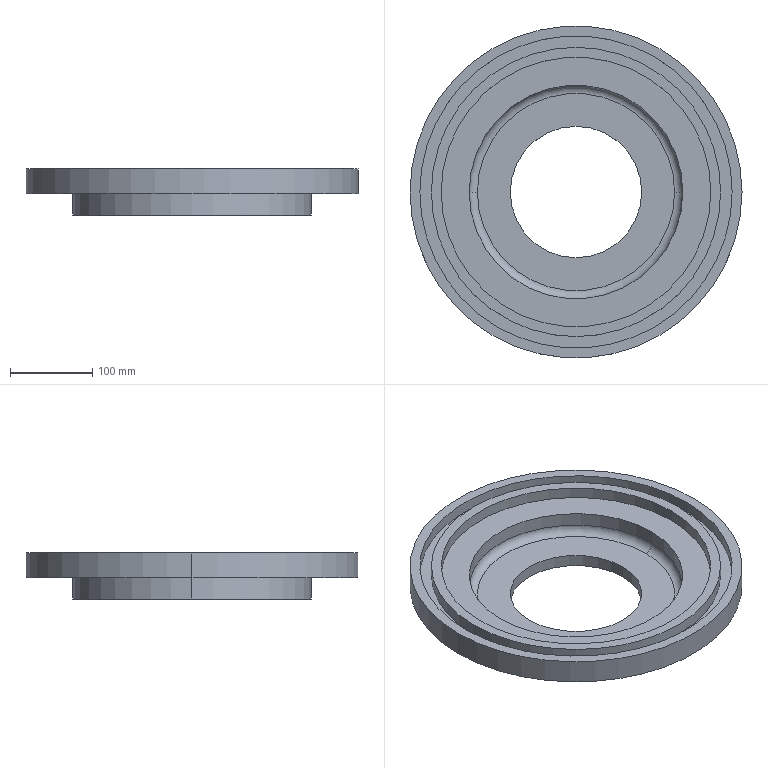Part | SolidWorks | features Fillet 1, Revolution 1 | 1 solid | 23 faces | box 404 x 404 x 56 mm | volume 2436851 mm3 | cylinder 14 | plane 7 | torus 2 | commonest cylinder face diameters 160 x2 260 x2 290 x2 328 x2 352 x2 380 x2
STEP:
#1=CARTESIAN_POINT('',(130.,0.,-31.));
#2=VERTEX_POINT('',#1);
#3=CARTESIAN_POINT('',(-130.,0.,-31.));
#4=VERTEX_POINT('',#3);
#5=CARTESIAN_POINT('',(0.,0.,-31.));
#6=DIRECTION('',(0.,0.,-1.));
#7=DIRECTION('',(-1.,0.,0.));
#8=AXIS2_PLACEMENT_3D('',#5,#6,#7);
#9=CIRCLE('',#8,130.);
#10=EDGE_CURVE('',#2,#4,#9,.T.);
#11=ORIENTED_EDGE('',*,*,#10,.F.);
#12=CARTESIAN_POINT('',(120.,0.,-41.));
#13=VERTEX_POINT('',#12);
#14=CARTESIAN_POINT('',(120.,0.,-31.));
#15=DIRECTION('',(0.,1.,0.));
#16=DIRECTION('',(-1.,0.,0.));
#17=AXIS2_PLACEMENT_3D('',#14,#15,#16);
#18=CIRCLE('',#17,10.);
#19=EDGE_CURVE('',#2,#13,#18,.T.);
#20=ORIENTED_EDGE('',*,*,#19,.T.);
#21=CARTESIAN_POINT('',(-120.,0.,-41.));
#22=VERTEX_POINT('',#21);
#23=CARTESIAN_POINT('',(0.,0.,-41.));
#24=DIRECTION('',(0.,0.,1.));
#25=DIRECTION('',(-1.,0.,0.));
#26=AXIS2_PLACEMENT_3D('',#23,#24,#25);
#27=CIRCLE('',#26,120.);
#28=EDGE_CURVE('',#22,#13,#27,.T.);
#29=ORIENTED_EDGE('',*,*,#28,.F.);
#30=CARTESIAN_POINT('',(-120.,0.,-31.));
#31=DIRECTION('',(0.,-1.,0.));
#32=DIRECTION('',(0.,0.,-1.));
#33=AXIS2_PLACEMENT_3D('',#30,#31,#32);
#34=CIRCLE('',#33,10.);
#35=EDGE_CURVE('',#4,#22,#34,.T.);
#36=ORIENTED_EDGE('',*,*,#35,.F.);
#37=EDGE_LOOP('',(#11,#20,#29,#36));
#38=FACE_OUTER_BOUND('',#37,.T.);
#39=CARTESIAN_POINT('',(0.,0.,-31.));
#40=DIRECTION('',(0.,0.,-1.));
#41=DIRECTION('',(-1.,0.,0.));
#42=AXIS2_PLACEMENT_3D('',#39,#40,#41);
#43=TOROIDAL_SURFACE('',#42,120.,10.);
#44=ADVANCED_FACE('',(#38),#43,.F.);
#45=CARTESIAN_POINT('',(-190.,0.,-14.));
#46=VERTEX_POINT('',#45);
#47=CARTESIAN_POINT('',(190.,0.,-14.));
#48=VERTEX_POINT('',#47);
#49=CARTESIAN_POINT('',(0.,0.,-14.));
#50=DIRECTION('',(0.,0.,1.));
#51=DIRECTION('',(1.,0.,0.));
#52=AXIS2_PLACEMENT_3D('',#49,#50,#51);
#53=CIRCLE('',#52,190.);
#54=EDGE_CURVE('',#46,#48,#53,.T.);
#55=ORIENTED_EDGE('',*,*,#54,.F.);
#56=CARTESIAN_POINT('',(-190.,0.,0.));
#57=VERTEX_POINT('',#56);
#58=CARTESIAN_POINT('',(-190.,0.,0.));
#59=DIRECTION('',(0.,0.,1.));
#60=VECTOR('',#59,1000.);
#61=LINE('',#58,#60);
#62=EDGE_CURVE('',#46,#57,#61,.T.);
#63=ORIENTED_EDGE('',*,*,#62,.T.);
#64=CARTESIAN_POINT('',(190.,0.,0.));
#65=VERTEX_POINT('',#64);
#66=CARTESIAN_POINT('',(0.,0.,0.));
#67=DIRECTION('',(0.,0.,1.));
#68=DIRECTION('',(1.,0.,0.));
#69=AXIS2_PLACEMENT_3D('',#66,#67,#68);
#70=CIRCLE('',#69,190.);
#71=EDGE_CURVE('',#57,#65,#70,.T.);
#72=ORIENTED_EDGE('',*,*,#71,.T.);
#73=CARTESIAN_POINT('',(190.,0.,0.));
#74=DIRECTION('',(0.,0.,1.));
#75=VECTOR('',#74,1000.);
#76=LINE('',#73,#75);
#77=EDGE_CURVE('',#48,#65,#76,.T.);
#78=ORIENTED_EDGE('',*,*,#77,.F.);
#79=EDGE_LOOP('',(#55,#63,#72,#78));
#80=FACE_OUTER_BOUND('',#79,.T.);
#81=CARTESIAN_POINT('',(0.,0.,0.));
#82=DIRECTION('',(0.,0.,1.));
#83=DIRECTION('',(1.,0.,0.));
#84=AXIS2_PLACEMENT_3D('',#81,#82,#83);
#85=CYLINDRICAL_SURFACE('',#84,190.);
#86=ADVANCED_FACE('',(#80),#85,.F.);
#87=CARTESIAN_POINT('',(176.,0.,-14.));
#88=VERTEX_POINT('',#87);
#89=CARTESIAN_POINT('',(-176.,0.,-14.));
#90=VERTEX_POINT('',#89);
#91=CARTESIAN_POINT('',(0.,0.,-14.));
#92=DIRECTION('',(0.,0.,1.));
#93=DIRECTION('',(1.,0.,0.));
#94=AXIS2_PLACEMENT_3D('',#91,#92,#93);
#95=CIRCLE('',#94,176.);
#96=EDGE_CURVE('',#88,#90,#95,.T.);
#97=ORIENTED_EDGE('',*,*,#96,.T.);
#98=CARTESIAN_POINT('',(-176.,0.,0.));
#99=VERTEX_POINT('',#98);
#100=CARTESIAN_POINT('',(-176.,0.,0.));
#101=DIRECTION('',(0.,0.,1.));
#102=VECTOR('',#101,1000.);
#103=LINE('',#100,#102);
#104=EDGE_CURVE('',#90,#99,#103,.T.);
#105=ORIENTED_EDGE('',*,*,#104,.T.);
#106=CARTESIAN_POINT('',(176.,0.,0.));
#107=VERTEX_POINT('',#106);
#108=CARTESIAN_POINT('',(0.,0.,0.));
#109=DIRECTION('',(0.,0.,1.));
#110=DIRECTION('',(1.,0.,0.));
#111=AXIS2_PLACEMENT_3D('',#108,#109,#110);
#112=CIRCLE('',#111,176.);
#113=EDGE_CURVE('',#107,#99,#112,.T.);
#114=ORIENTED_EDGE('',*,*,#113,.F.);
#115=CARTESIAN_POINT('',(176.,0.,0.));
#116=DIRECTION('',(0.,0.,1.));
#117=VECTOR('',#116,1000.);
#118=LINE('',#115,#117);
#119=EDGE_CURVE('',#88,#107,#118,.T.);
#120=ORIENTED_EDGE('',*,*,#119,.F.);
#121=EDGE_LOOP('',(#97,#105,#114,#120));
#122=FACE_OUTER_BOUND('',#121,.T.);
#123=CARTESIAN_POINT('',(0.,0.,0.));
#124=DIRECTION('',(0.,0.,1.));
#125=DIRECTION('',(1.,0.,0.));
#126=AXIS2_PLACEMENT_3D('',#123,#124,#125);
#127=CYLINDRICAL_SURFACE('',#126,176.);
#128=ADVANCED_FACE('',(#122),#127,.T.);
#129=CARTESIAN_POINT('',(-164.,0.,-14.));
#130=VERTEX_POINT('',#129);
#131=CARTESIAN_POINT('',(164.,0.,-14.));
#132=VERTEX_POINT('',#131);
#133=CARTESIAN_POINT('',(0.,0.,-14.));
#134=DIRECTION('',(0.,0.,1.));
#135=DIRECTION('',(1.,0.,0.));
#136=AXIS2_PLACEMENT_3D('',#133,#134,#135);
#137=CIRCLE('',#136,164.);
#138=EDGE_CURVE('',#130,#132,#137,.T.);
#139=ORIENTED_EDGE('',*,*,#138,.F.);
#140=CARTESIAN_POINT('',(-164.,0.,0.));
#141=VERTEX_POINT('',#140);
#142=CARTESIAN_POINT('',(-164.,0.,0.));
#143=DIRECTION('',(0.,0.,1.));
#144=VECTOR('',#143,1000.);
#145=LINE('',#142,#144);
#146=EDGE_CURVE('',#130,#141,#145,.T.);
#147=ORIENTED_EDGE('',*,*,#146,.T.);
#148=CARTESIAN_POINT('',(164.,0.,0.));
#149=VERTEX_POINT('',#148);
#150=CARTESIAN_POINT('',(0.,0.,0.));
#151=DIRECTION('',(0.,0.,1.));
#152=DIRECTION('',(1.,0.,0.));
#153=AXIS2_PLACEMENT_3D('',#150,#151,#152);
#154=CIRCLE('',#153,164.);
#155=EDGE_CURVE('',#141,#149,#154,.T.);
#156=ORIENTED_EDGE('',*,*,#155,.T.);
#157=CARTESIAN_POINT('',(164.,0.,0.));
#158=DIRECTION('',(0.,0.,1.));
#159=VECTOR('',#158,1000.);
#160=LINE('',#157,#159);
#161=EDGE_CURVE('',#132,#149,#160,.T.);
#162=ORIENTED_EDGE('',*,*,#161,.F.);
#163=EDGE_LOOP('',(#139,#147,#156,#162));
#164=FACE_OUTER_BOUND('',#163,.T.);
#165=CARTESIAN_POINT('',(0.,0.,0.));
#166=DIRECTION('',(0.,0.,1.));
#167=DIRECTION('',(1.,0.,0.));
#168=AXIS2_PLACEMENT_3D('',#165,#166,#167);
#169=CYLINDRICAL_SURFACE('',#168,164.);
#170=ADVANCED_FACE('',(#164),#169,.F.);
#171=ORIENTED_EDGE('',*,*,#10,.T.);
#172=CARTESIAN_POINT('',(-130.,0.,-14.));
#173=VERTEX_POINT('',#172);
#174=CARTESIAN_POINT('',(-130.,0.,0.));
#175=DIRECTION('',(0.,0.,1.));
#176=VECTOR('',#175,1000.);
#177=LINE('',#174,#176);
#178=EDGE_CURVE('',#4,#173,#177,.T.);
#179=ORIENTED_EDGE('',*,*,#178,.T.);
#180=CARTESIAN_POINT('',(130.,0.,-14.));
#181=VERTEX_POINT('',#180);
#182=CARTESIAN_POINT('',(0.,0.,-14.));
#183=DIRECTION('',(0.,0.,1.));
#184=DIRECTION('',(1.,0.,0.));
#185=AXIS2_PLACEMENT_3D('',#182,#183,#184);
#186=CIRCLE('',#185,130.);
#187=EDGE_CURVE('',#173,#181,#186,.T.);
#188=ORIENTED_EDGE('',*,*,#187,.T.);
#189=CARTESIAN_POINT('',(130.,0.,0.));
#190=DIRECTION('',(0.,0.,1.));
#191=VECTOR('',#190,1000.);
#192=LINE('',#189,#191);
#193=EDGE_CURVE('',#2,#181,#192,.T.);
#194=ORIENTED_EDGE('',*,*,#193,.F.);
#195=EDGE_LOOP('',(#171,#179,#188,#194));
#196=FACE_OUTER_BOUND('',#195,.T.);
#197=CARTESIAN_POINT('',(0.,0.,0.));
#198=DIRECTION('',(0.,0.,1.));
#199=DIRECTION('',(1.,0.,0.));
#200=AXIS2_PLACEMENT_3D('',#197,#198,#199);
#201=CYLINDRICAL_SURFACE('',#200,130.);
#202=ADVANCED_FACE('',(#196),#201,.F.);
#203=CARTESIAN_POINT('',(-80.,0.,-56.));
#204=VERTEX_POINT('',#203);
#205=CARTESIAN_POINT('',(80.,0.,-56.));
#206=VERTEX_POINT('',#205);
#207=CARTESIAN_POINT('',(0.,0.,-56.));
#208=DIRECTION('',(0.,0.,1.));
#209=DIRECTION('',(1.,0.,0.));
#210=AXIS2_PLACEMENT_3D('',#207,#208,#209);
#211=CIRCLE('',#210,80.);
#212=EDGE_CURVE('',#204,#206,#211,.T.);
#213=ORIENTED_EDGE('',*,*,#212,.F.);
#214=CARTESIAN_POINT('',(-80.,0.,-41.));
#215=VERTEX_POINT('',#214);
#216=CARTESIAN_POINT('',(-80.,0.,0.));
#217=DIRECTION('',(0.,0.,1.));
#218=VECTOR('',#217,1000.);
#219=LINE('',#216,#218);
#220=EDGE_CURVE('',#204,#215,#219,.T.);
#221=ORIENTED_EDGE('',*,*,#220,.T.);
#222=CARTESIAN_POINT('',(80.,0.,-41.));
#223=VERTEX_POINT('',#222);
#224=CARTESIAN_POINT('',(0.,0.,-41.));
#225=DIRECTION('',(0.,0.,1.));
#226=DIRECTION('',(1.,0.,0.));
#227=AXIS2_PLACEMENT_3D('',#224,#225,#226);
#228=CIRCLE('',#227,80.);
#229=EDGE_CURVE('',#215,#223,#228,.T.);
#230=ORIENTED_EDGE('',*,*,#229,.T.);
#231=CARTESIAN_POINT('',(80.,0.,0.));
#232=DIRECTION('',(0.,0.,1.));
#233=VECTOR('',#232,1000.);
#234=LINE('',#231,#233);
#235=EDGE_CURVE('',#206,#223,#234,.T.);
#236=ORIENTED_EDGE('',*,*,#235,.F.);
#237=EDGE_LOOP('',(#213,#221,#230,#236));
#238=FACE_OUTER_BOUND('',#237,.T.);
#239=CARTESIAN_POINT('',(0.,0.,0.));
#240=DIRECTION('',(0.,0.,1.));
#241=DIRECTION('',(1.,0.,0.));
#242=AXIS2_PLACEMENT_3D('',#239,#240,#241);
#243=CYLINDRICAL_SURFACE('',#242,80.);
#244=ADVANCED_FACE('',(#238),#243,.F.);
#245=CARTESIAN_POINT('',(145.,0.,-56.));
#246=VERTEX_POINT('',#245);
#247=CARTESIAN_POINT('',(-145.,0.,-56.));
#248=VERTEX_POINT('',#247);
#249=CARTESIAN_POINT('',(0.,0.,-56.));
#250=DIRECTION('',(0.,0.,1.));
#251=DIRECTION('',(1.,0.,0.));
#252=AXIS2_PLACEMENT_3D('',#249,#250,#251);
#253=CIRCLE('',#252,145.);
#254=EDGE_CURVE('',#246,#248,#253,.T.);
#255=ORIENTED_EDGE('',*,*,#254,.T.);
#256=CARTESIAN_POINT('',(-145.,0.,-30.));
#257=VERTEX_POINT('',#256);
#258=CARTESIAN_POINT('',(-145.,0.,0.));
#259=DIRECTION('',(0.,0.,1.));
#260=VECTOR('',#259,1000.);
#261=LINE('',#258,#260);
#262=EDGE_CURVE('',#248,#257,#261,.T.);
#263=ORIENTED_EDGE('',*,*,#262,.T.);
#264=CARTESIAN_POINT('',(145.,0.,-30.));
#265=VERTEX_POINT('',#264);
#266=CARTESIAN_POINT('',(0.,0.,-30.));
#267=DIRECTION('',(0.,0.,1.));
#268=DIRECTION('',(1.,0.,0.));
#269=AXIS2_PLACEMENT_3D('',#266,#267,#268);
#270=CIRCLE('',#269,145.);
#271=EDGE_CURVE('',#265,#257,#270,.T.);
#272=ORIENTED_EDGE('',*,*,#271,.F.);
#273=CARTESIAN_POINT('',(145.,0.,0.));
#274=DIRECTION('',(0.,0.,1.));
#275=VECTOR('',#274,1000.);
#276=LINE('',#273,#275);
#277=EDGE_CURVE('',#246,#265,#276,.T.);
#278=ORIENTED_EDGE('',*,*,#277,.F.);
#279=EDGE_LOOP('',(#255,#263,#272,#278));
#280=FACE_OUTER_BOUND('',#279,.T.);
#281=CARTESIAN_POINT('',(0.,0.,0.));
#282=DIRECTION('',(0.,0.,1.));
#283=DIRECTION('',(1.,0.,0.));
#284=AXIS2_PLACEMENT_3D('',#281,#282,#283);
#285=CYLINDRICAL_SURFACE('',#284,145.);
#286=ADVANCED_FACE('',(#280),#285,.T.);
#287=CARTESIAN_POINT('',(202.,0.,-30.));
#288=VERTEX_POINT('',#287);
#289=CARTESIAN_POINT('',(-202.,0.,-30.));
#290=VERTEX_POINT('',#289);
#291=CARTESIAN_POINT('',(0.,0.,-30.));
#292=DIRECTION('',(0.,0.,1.));
#293=DIRECTION('',(1.,0.,0.));
#294=AXIS2_PLACEMENT_3D('',#291,#292,#293);
#295=CIRCLE('',#294,202.);
#296=EDGE_CURVE('',#288,#290,#295,.T.);
#297=ORIENTED_EDGE('',*,*,#296,.T.);
#298=CARTESIAN_POINT('',(-202.,0.,0.));
#299=VERTEX_POINT('',#298);
#300=CARTESIAN_POINT('',(-202.,0.,0.));
#301=DIRECTION('',(0.,0.,1.));
#302=VECTOR('',#301,1000.);
#303=LINE('',#300,#302);
#304=EDGE_CURVE('',#290,#299,#303,.T.);
#305=ORIENTED_EDGE('',*,*,#304,.T.);
#306=CARTESIAN_POINT('',(202.,0.,0.));
#307=VERTEX_POINT('',#306);
#308=CARTESIAN_POINT('',(0.,0.,0.));
#309=DIRECTION('',(0.,0.,1.));
#310=DIRECTION('',(1.,0.,0.));
#311=AXIS2_PLACEMENT_3D('',#308,#309,#310);
#312=CIRCLE('',#311,202.);
#313=EDGE_CURVE('',#307,#299,#312,.T.);
#314=ORIENTED_EDGE('',*,*,#313,.F.);
#315=CARTESIAN_POINT('',(202.,0.,0.));
#316=DIRECTION('',(0.,0.,1.));
#317=VECTOR('',#316,1000.);
#318=LINE('',#315,#317);
#319=EDGE_CURVE('',#288,#307,#318,.T.);
#320=ORIENTED_EDGE('',*,*,#319,.F.);
#321=EDGE_LOOP('',(#297,#305,#314,#320));
#322=FACE_OUTER_BOUND('',#321,.T.);
#323=CARTESIAN_POINT('',(0.,0.,0.));
#324=DIRECTION('',(0.,0.,1.));
#325=DIRECTION('',(1.,0.,0.));
#326=AXIS2_PLACEMENT_3D('',#323,#324,#325);
#327=CYLINDRICAL_SURFACE('',#326,202.);
#328=ADVANCED_FACE('',(#322),#327,.T.);
#329=CARTESIAN_POINT('',(0.,0.,0.));
#330=DIRECTION('',(0.,0.,1.));
#331=DIRECTION('',(1.,0.,0.));
#332=AXIS2_PLACEMENT_3D('',#329,#330,#331);
#333=CIRCLE('',#332,190.);
#334=EDGE_CURVE('',#65,#57,#333,.T.);
#335=ORIENTED_EDGE('',*,*,#334,.F.);
#336=ORIENTED_EDGE('',*,*,#71,.F.);
#337=EDGE_LOOP('',(#335,#336));
#338=FACE_BOUND('',#337,.T.);
#339=ORIENTED_EDGE('',*,*,#313,.T.);
#340=CARTESIAN_POINT('',(0.,0.,0.));
#341=DIRECTION('',(0.,0.,1.));
#342=DIRECTION('',(1.,0.,0.));
#343=AXIS2_PLACEMENT_3D('',#340,#341,#342);
#344=CIRCLE('',#343,202.);
#345=EDGE_CURVE('',#299,#307,#344,.T.);
#346=ORIENTED_EDGE('',*,*,#345,.T.);
#347=EDGE_LOOP('',(#339,#346));
#348=FACE_OUTER_BOUND('',#347,.T.);
#349=CARTESIAN_POINT('',(0.,190.,0.));
#350=DIRECTION('',(0.,0.,-1.));
#351=DIRECTION('',(-1.,0.,0.));
#352=AXIS2_PLACEMENT_3D('',#349,#350,#351);
#353=PLANE('',#352);
#354=ADVANCED_FACE('',(#338,#348),#353,.F.);
#355=ORIENTED_EDGE('',*,*,#304,.F.);
#356=CARTESIAN_POINT('',(0.,0.,-30.));
#357=DIRECTION('',(0.,0.,1.));
#358=DIRECTION('',(1.,0.,0.));
#359=AXIS2_PLACEMENT_3D('',#356,#357,#358);
#360=CIRCLE('',#359,202.);
#361=EDGE_CURVE('',#290,#288,#360,.T.);
#362=ORIENTED_EDGE('',*,*,#361,.T.);
#363=ORIENTED_EDGE('',*,*,#319,.T.);
#364=ORIENTED_EDGE('',*,*,#345,.F.);
#365=EDGE_LOOP('',(#355,#362,#363,#364));
#366=FACE_OUTER_BOUND('',#365,.T.);
#367=CARTESIAN_POINT('',(0.,0.,0.));
#368=DIRECTION('',(0.,0.,1.));
#369=DIRECTION('',(1.,0.,0.));
#370=AXIS2_PLACEMENT_3D('',#367,#368,#369);
#371=CYLINDRICAL_SURFACE('',#370,202.);
#372=ADVANCED_FACE('',(#366),#371,.T.);
#373=ORIENTED_EDGE('',*,*,#296,.F.);
#374=ORIENTED_EDGE('',*,*,#361,.F.);
#375=EDGE_LOOP('',(#373,#374));
#376=FACE_OUTER_BOUND('',#375,.T.);
#377=ORIENTED_EDGE('',*,*,#271,.T.);
#378=CARTESIAN_POINT('',(0.,0.,-30.));
#379=DIRECTION('',(0.,0.,1.));
#380=DIRECTION('',(1.,0.,0.));
#381=AXIS2_PLACEMENT_3D('',#378,#379,#380);
#382=CIRCLE('',#381,145.);
#383=EDGE_CURVE('',#257,#265,#382,.T.);
#384=ORIENTED_EDGE('',*,*,#383,.T.);
#385=EDGE_LOOP('',(#377,#384));
#386=FACE_BOUND('',#385,.T.);
#387=CARTESIAN_POINT('',(0.,202.,-30.));
#388=DIRECTION('',(0.,0.,1.));
#389=DIRECTION('',(1.,0.,0.));
#390=AXIS2_PLACEMENT_3D('',#387,#388,#389);
#391=PLANE('',#390);
#392=ADVANCED_FACE('',(#376,#386),#391,.F.);
#393=ORIENTED_EDGE('',*,*,#262,.F.);
#394=CARTESIAN_POINT('',(0.,0.,-56.));
#395=DIRECTION('',(0.,0.,1.));
#396=DIRECTION('',(1.,0.,0.));
#397=AXIS2_PLACEMENT_3D('',#394,#395,#396);
#398=CIRCLE('',#397,145.);
#399=EDGE_CURVE('',#248,#246,#398,.T.);
#400=ORIENTED_EDGE('',*,*,#399,.T.);
#401=ORIENTED_EDGE('',*,*,#277,.T.);
#402=ORIENTED_EDGE('',*,*,#383,.F.);
#403=EDGE_LOOP('',(#393,#400,#401,#402));
#404=FACE_OUTER_BOUND('',#403,.T.);
#405=CARTESIAN_POINT('',(0.,0.,0.));
#406=DIRECTION('',(0.,0.,1.));
#407=DIRECTION('',(1.,0.,0.));
#408=AXIS2_PLACEMENT_3D('',#405,#406,#407);
#409=CYLINDRICAL_SURFACE('',#408,145.);
#410=ADVANCED_FACE('',(#404),#409,.T.);
#411=ORIENTED_EDGE('',*,*,#254,.F.);
#412=ORIENTED_EDGE('',*,*,#399,.F.);
#413=EDGE_LOOP('',(#411,#412));
#414=FACE_OUTER_BOUND('',#413,.T.);
#415=CARTESIAN_POINT('',(0.,0.,-56.));
#416=DIRECTION('',(0.,0.,1.));
#417=DIRECTION('',(1.,0.,0.));
#418=AXIS2_PLACEMENT_3D('',#415,#416,#417);
#419=CIRCLE('',#418,80.);
#420=EDGE_CURVE('',#206,#204,#419,.T.);
#421=ORIENTED_EDGE('',*,*,#420,.T.);
#422=ORIENTED_EDGE('',*,*,#212,.T.);
#423=EDGE_LOOP('',(#421,#422));
#424=FACE_BOUND('',#423,.T.);
#425=CARTESIAN_POINT('',(0.,145.,-56.));
#426=DIRECTION('',(0.,0.,1.));
#427=DIRECTION('',(1.,0.,0.));
#428=AXIS2_PLACEMENT_3D('',#425,#426,#427);
#429=PLANE('',#428);
#430=ADVANCED_FACE('',(#414,#424),#429,.F.);
#431=ORIENTED_EDGE('',*,*,#220,.F.);
#432=ORIENTED_EDGE('',*,*,#420,.F.);
#433=ORIENTED_EDGE('',*,*,#235,.T.);
#434=CARTESIAN_POINT('',(0.,0.,-41.));
#435=DIRECTION('',(0.,0.,1.));
#436=DIRECTION('',(1.,0.,0.));
#437=AXIS2_PLACEMENT_3D('',#434,#435,#436);
#438=CIRCLE('',#437,80.);
#439=EDGE_CURVE('',#223,#215,#438,.T.);
#440=ORIENTED_EDGE('',*,*,#439,.T.);
#441=EDGE_LOOP('',(#431,#432,#433,#440));
#442=FACE_OUTER_BOUND('',#441,.T.);
#443=CARTESIAN_POINT('',(0.,0.,0.));
#444=DIRECTION('',(0.,0.,1.));
#445=DIRECTION('',(1.,0.,0.));
#446=AXIS2_PLACEMENT_3D('',#443,#444,#445);
#447=CYLINDRICAL_SURFACE('',#446,80.);
#448=ADVANCED_FACE('',(#442),#447,.F.);
#449=ORIENTED_EDGE('',*,*,#28,.T.);
#450=CARTESIAN_POINT('',(0.,0.,-41.));
#451=DIRECTION('',(0.,0.,1.));
#452=DIRECTION('',(-1.,0.,0.));
#453=AXIS2_PLACEMENT_3D('',#450,#451,#452);
#454=CIRCLE('',#453,120.);
#455=EDGE_CURVE('',#13,#22,#454,.T.);
#456=ORIENTED_EDGE('',*,*,#455,.T.);
#457=EDGE_LOOP('',(#449,#456));
#458=FACE_OUTER_BOUND('',#457,.T.);
#459=ORIENTED_EDGE('',*,*,#439,.F.);
#460=ORIENTED_EDGE('',*,*,#229,.F.);
#461=EDGE_LOOP('',(#459,#460));
#462=FACE_BOUND('',#461,.T.);
#463=CARTESIAN_POINT('',(0.,80.,-41.));
#464=DIRECTION('',(0.,0.,-1.));
#465=DIRECTION('',(-1.,0.,0.));
#466=AXIS2_PLACEMENT_3D('',#463,#464,#465);
#467=PLANE('',#466);
#468=ADVANCED_FACE('',(#458,#462),#467,.F.);
#469=ORIENTED_EDGE('',*,*,#178,.F.);
#470=CARTESIAN_POINT('',(0.,0.,-31.));
#471=DIRECTION('',(0.,0.,-1.));
#472=DIRECTION('',(-1.,0.,0.));
#473=AXIS2_PLACEMENT_3D('',#470,#471,#472);
#474=CIRCLE('',#473,130.);
#475=EDGE_CURVE('',#4,#2,#474,.T.);
#476=ORIENTED_EDGE('',*,*,#475,.T.);
#477=ORIENTED_EDGE('',*,*,#193,.T.);
#478=CARTESIAN_POINT('',(0.,0.,-14.));
#479=DIRECTION('',(0.,0.,1.));
#480=DIRECTION('',(1.,0.,0.));
#481=AXIS2_PLACEMENT_3D('',#478,#479,#480);
#482=CIRCLE('',#481,130.);
#483=EDGE_CURVE('',#181,#173,#482,.T.);
#484=ORIENTED_EDGE('',*,*,#483,.T.);
#485=EDGE_LOOP('',(#469,#476,#477,#484));
#486=FACE_OUTER_BOUND('',#485,.T.);
#487=CARTESIAN_POINT('',(0.,0.,0.));
#488=DIRECTION('',(0.,0.,1.));
#489=DIRECTION('',(1.,0.,0.));
#490=AXIS2_PLACEMENT_3D('',#487,#488,#489);
#491=CYLINDRICAL_SURFACE('',#490,130.);
#492=ADVANCED_FACE('',(#486),#491,.F.);
#493=ORIENTED_EDGE('',*,*,#483,.F.);
#494=ORIENTED_EDGE('',*,*,#187,.F.);
#495=EDGE_LOOP('',(#493,#494));
#496=FACE_BOUND('',#495,.T.);
#497=CARTESIAN_POINT('',(0.,0.,-14.));
#498=DIRECTION('',(0.,0.,1.));
#499=DIRECTION('',(1.,0.,0.));
#500=AXIS2_PLACEMENT_3D('',#497,#498,#499);
#501=CIRCLE('',#500,164.);
#502=EDGE_CURVE('',#132,#130,#501,.T.);
#503=ORIENTED_EDGE('',*,*,#502,.T.);
#504=ORIENTED_EDGE('',*,*,#138,.T.);
#505=EDGE_LOOP('',(#503,#504));
#506=FACE_OUTER_BOUND('',#505,.T.);
#507=CARTESIAN_POINT('',(0.,130.,-14.));
#508=DIRECTION('',(0.,0.,-1.));
#509=DIRECTION('',(-1.,0.,0.));
#510=AXIS2_PLACEMENT_3D('',#507,#508,#509);
#511=PLANE('',#510);
#512=ADVANCED_FACE('',(#496,#506),#511,.F.);
#513=ORIENTED_EDGE('',*,*,#146,.F.);
#514=ORIENTED_EDGE('',*,*,#502,.F.);
#515=ORIENTED_EDGE('',*,*,#161,.T.);
#516=CARTESIAN_POINT('',(0.,0.,0.));
#517=DIRECTION('',(0.,0.,1.));
#518=DIRECTION('',(1.,0.,0.));
#519=AXIS2_PLACEMENT_3D('',#516,#517,#518);
#520=CIRCLE('',#519,164.);
#521=EDGE_CURVE('',#149,#141,#520,.T.);
#522=ORIENTED_EDGE('',*,*,#521,.T.);
#523=EDGE_LOOP('',(#513,#514,#515,#522));
#524=FACE_OUTER_BOUND('',#523,.T.);
#525=CARTESIAN_POINT('',(0.,0.,0.));
#526=DIRECTION('',(0.,0.,1.));
#527=DIRECTION('',(1.,0.,0.));
#528=AXIS2_PLACEMENT_3D('',#525,#526,#527);
#529=CYLINDRICAL_SURFACE('',#528,164.);
#530=ADVANCED_FACE('',(#524),#529,.F.);
#531=ORIENTED_EDGE('',*,*,#521,.F.);
#532=ORIENTED_EDGE('',*,*,#155,.F.);
#533=EDGE_LOOP('',(#531,#532));
#534=FACE_BOUND('',#533,.T.);
#535=ORIENTED_EDGE('',*,*,#113,.T.);
#536=CARTESIAN_POINT('',(0.,0.,0.));
#537=DIRECTION('',(0.,0.,1.));
#538=DIRECTION('',(1.,0.,0.));
#539=AXIS2_PLACEMENT_3D('',#536,#537,#538);
#540=CIRCLE('',#539,176.);
#541=EDGE_CURVE('',#99,#107,#540,.T.);
#542=ORIENTED_EDGE('',*,*,#541,.T.);
#543=EDGE_LOOP('',(#535,#542));
#544=FACE_OUTER_BOUND('',#543,.T.);
#545=CARTESIAN_POINT('',(0.,164.,0.));
#546=DIRECTION('',(0.,0.,-1.));
#547=DIRECTION('',(-1.,0.,0.));
#548=AXIS2_PLACEMENT_3D('',#545,#546,#547);
#549=PLANE('',#548);
#550=ADVANCED_FACE('',(#534,#544),#549,.F.);
#551=ORIENTED_EDGE('',*,*,#104,.F.);
#552=CARTESIAN_POINT('',(0.,0.,-14.));
#553=DIRECTION('',(0.,0.,1.));
#554=DIRECTION('',(1.,0.,0.));
#555=AXIS2_PLACEMENT_3D('',#552,#553,#554);
#556=CIRCLE('',#555,176.);
#557=EDGE_CURVE('',#90,#88,#556,.T.);
#558=ORIENTED_EDGE('',*,*,#557,.T.);
#559=ORIENTED_EDGE('',*,*,#119,.T.);
#560=ORIENTED_EDGE('',*,*,#541,.F.);
#561=EDGE_LOOP('',(#551,#558,#559,#560));
#562=FACE_OUTER_BOUND('',#561,.T.);
#563=CARTESIAN_POINT('',(0.,0.,0.));
#564=DIRECTION('',(0.,0.,1.));
#565=DIRECTION('',(1.,0.,0.));
#566=AXIS2_PLACEMENT_3D('',#563,#564,#565);
#567=CYLINDRICAL_SURFACE('',#566,176.);
#568=ADVANCED_FACE('',(#562),#567,.T.);
#569=ORIENTED_EDGE('',*,*,#96,.F.);
#570=ORIENTED_EDGE('',*,*,#557,.F.);
#571=EDGE_LOOP('',(#569,#570));
#572=FACE_BOUND('',#571,.T.);
#573=CARTESIAN_POINT('',(0.,0.,-14.));
#574=DIRECTION('',(0.,0.,1.));
#575=DIRECTION('',(1.,0.,0.));
#576=AXIS2_PLACEMENT_3D('',#573,#574,#575);
#577=CIRCLE('',#576,190.);
#578=EDGE_CURVE('',#48,#46,#577,.T.);
#579=ORIENTED_EDGE('',*,*,#578,.T.);
#580=ORIENTED_EDGE('',*,*,#54,.T.);
#581=EDGE_LOOP('',(#579,#580));
#582=FACE_OUTER_BOUND('',#581,.T.);
#583=CARTESIAN_POINT('',(0.,190.,-14.));
#584=DIRECTION('',(0.,0.,-1.));
#585=DIRECTION('',(-1.,0.,0.));
#586=AXIS2_PLACEMENT_3D('',#583,#584,#585);
#587=PLANE('',#586);
#588=ADVANCED_FACE('',(#572,#582),#587,.F.);
#589=ORIENTED_EDGE('',*,*,#62,.F.);
#590=ORIENTED_EDGE('',*,*,#578,.F.);
#591=ORIENTED_EDGE('',*,*,#77,.T.);
#592=ORIENTED_EDGE('',*,*,#334,.T.);
#593=EDGE_LOOP('',(#589,#590,#591,#592));
#594=FACE_OUTER_BOUND('',#593,.T.);
#595=CARTESIAN_POINT('',(0.,0.,0.));
#596=DIRECTION('',(0.,0.,1.));
#597=DIRECTION('',(1.,0.,0.));
#598=AXIS2_PLACEMENT_3D('',#595,#596,#597);
#599=CYLINDRICAL_SURFACE('',#598,190.);
#600=ADVANCED_FACE('',(#594),#599,.F.);
#601=ORIENTED_EDGE('',*,*,#19,.F.);
#602=ORIENTED_EDGE('',*,*,#475,.F.);
#603=ORIENTED_EDGE('',*,*,#35,.T.);
#604=ORIENTED_EDGE('',*,*,#455,.F.);
#605=EDGE_LOOP('',(#601,#602,#603,#604));
#606=FACE_OUTER_BOUND('',#605,.T.);
#607=CARTESIAN_POINT('',(0.,0.,-31.));
#608=DIRECTION('',(0.,0.,-1.));
#609=DIRECTION('',(-1.,0.,0.));
#610=AXIS2_PLACEMENT_3D('',#607,#608,#609);
#611=TOROIDAL_SURFACE('',#610,120.,10.);
#612=ADVANCED_FACE('',(#606),#611,.F.);
#613=CLOSED_SHELL('',(#44,#86,#128,#170,#202,#244,#286,#328,#354,#372,#392,#410,#430,#448,#468,#492,#512,#530,#550,#568,#588,#600,#612));
#614=MANIFOLD_SOLID_BREP('',#613);
#615=CARTESIAN_POINT('',(0.,0.,0.));
#616=DIRECTION('',(0.,0.,1.));
#617=DIRECTION('',(1.,0.,0.));
#618=AXIS2_PLACEMENT_3D('',#615,#616,#617);
#619=(LENGTH_UNIT()NAMED_UNIT(*)SI_UNIT(.MILLI.,.METRE.));
#620=UNCERTAINTY_MEASURE_WITH_UNIT(LENGTH_MEASURE(0.00001),#619,'','');
#621=(NAMED_UNIT(*)PLANE_ANGLE_UNIT()SI_UNIT($,.RADIAN.));
#622=(NAMED_UNIT(*)SI_UNIT($,.STERADIAN.)SOLID_ANGLE_UNIT());
#623=(GEOMETRIC_REPRESENTATION_CONTEXT(3)GLOBAL_UNCERTAINTY_ASSIGNED_CONTEXT((#620))GLOBAL_UNIT_ASSIGNED_CONTEXT((#619,#621,#622))REPRESENTATION_CONTEXT('',''));
#624=ADVANCED_BREP_SHAPE_REPRESENTATION('',(#614,#618),#623);